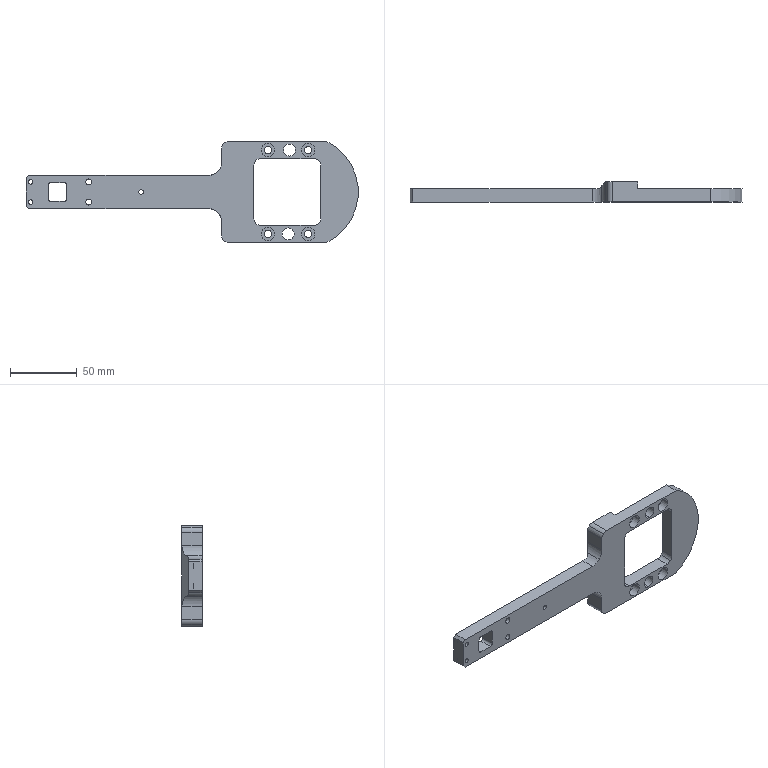Part | STEP file | ASND-0110-TPIM-022 | 1 solid | 89 faces | box 248.345 x 15 x 75.4 mm | volume 86870 mm3 | cylinder 59 | plane 30 | commonest cylinder face diameters 10 x20 5.5 x8 3.4 x6 4 x4 4.5 x4 6.5 x4